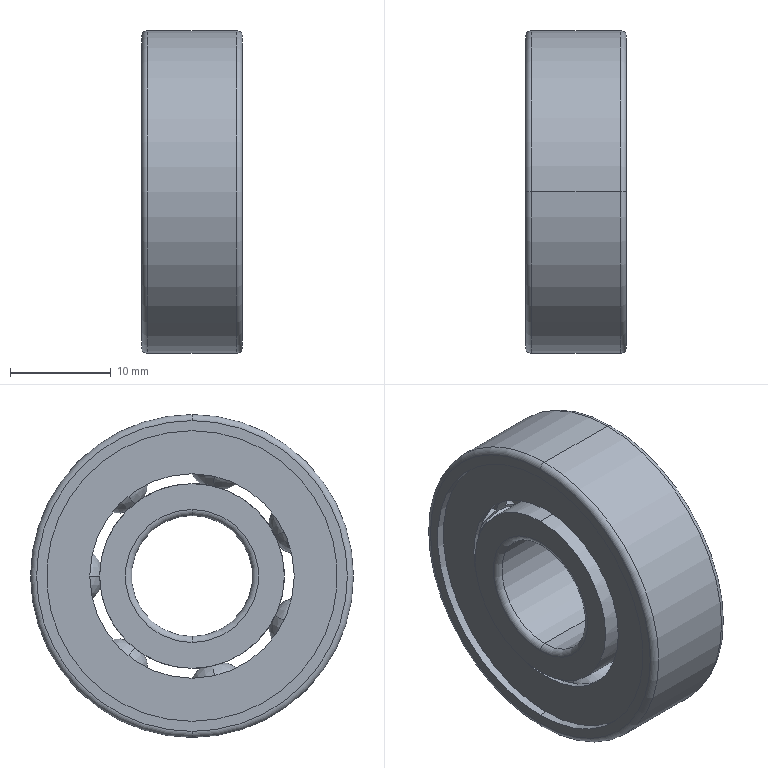Part | SolidWorks | features Revolution 6, CirPattern 2, RevCut 2, Cut 1, MirrorSolid 1 | 1 solid | 134 faces | box 10 x 32 x 32 mm | volume 4166 mm3 | sphere 56 | torus 32 | cylinder 24 | plane 22 | commonest cylinder face diameters 28.8 x8 18.3 x4 20.264 x4 12 x2 21.913 x2 25.187 x2